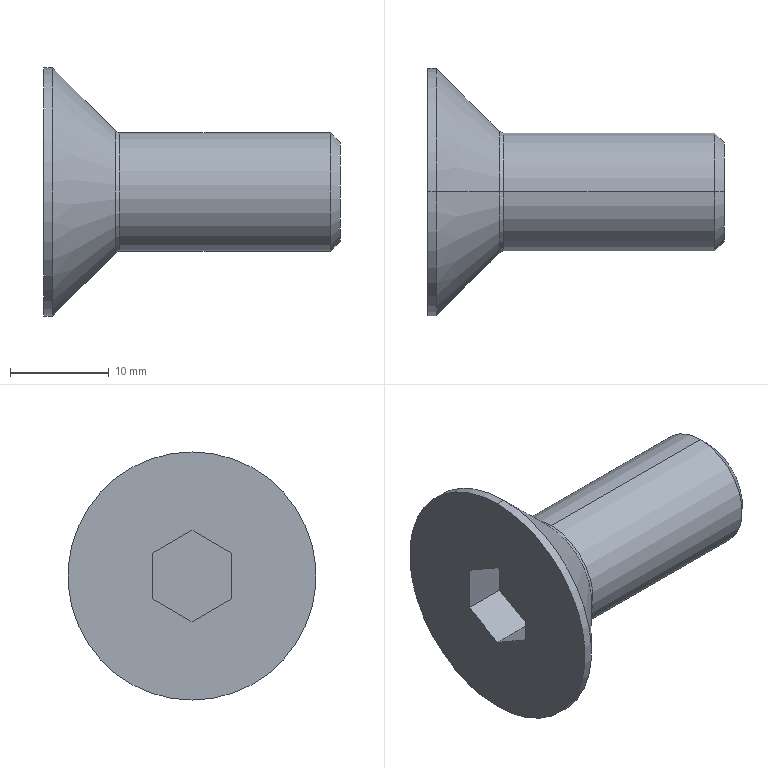Part | STEP file | 1 solid | 19 faces | box 30 x 25.075 x 25.075 mm | volume 4579 mm3 | plane 9 | cone 4 | cylinder 4 | spline 2 | commonest cylinder face diameters 12 x2 25.075 x2
STEP:
#1=CARTESIAN_POINT('',(0.,0.,0.));
#2=DIRECTION('',(0.,0.,1.));
#3=DIRECTION('',(1.,0.,0.));
#4=AXIS2_PLACEMENT_3D('',#1,#2,#3);
#5=CARTESIAN_POINT('',(22.56,0.,5.));
#6=VERTEX_POINT('',#5);
#7=CARTESIAN_POINT('',(22.56,0.,-5.));
#8=VERTEX_POINT('',#7);
#9=CARTESIAN_POINT('',(22.56,0.,0.));
#10=DIRECTION('',(-1.,0.,0.));
#11=DIRECTION('',(0.,0.,1.));
#12=AXIS2_PLACEMENT_3D('',#9,#10,#11);
#13=CIRCLE('',#12,5.);
#14=CARTESIAN_POINT('',(22.56,6.,0.));
#15=DIRECTION('',(-1.,0.,0.));
#16=DIRECTION('',(0.,0.,1.));
#17=AXIS2_PLACEMENT_3D('',#14,#15,#16);
#18=PLANE('',#17);
#19=CARTESIAN_POINT('',(0.,-6.));
#20=DIRECTION('',(1.,0.));
#21=AXIS2_PLACEMENT_2D('',#19,#20);
#22=CIRCLE('',#21,5.);
#23=(GEOMETRIC_REPRESENTATION_CONTEXT(2)PARAMETRIC_REPRESENTATION_CONTEXT()REPRESENTATION_CONTEXT('',''));
#24=DEFINITIONAL_REPRESENTATION('',(#22),#23);
#25=PCURVE('',#18,#24);
#26=CARTESIAN_POINT('',(21.56,0.,0.));
#27=DIRECTION('',(-1.,0.,0.));
#28=DIRECTION('',(0.,0.,1.));
#29=AXIS2_PLACEMENT_3D('',#26,#27,#28);
#30=CONICAL_SURFACE('',#29,6.,0.7854);
#31=CARTESIAN_POINT('',(0.,-1.));
#32=DIRECTION('',(1.,0.));
#33=VECTOR('',#32,1.);
#34=LINE('',#31,#33);
#35=(GEOMETRIC_REPRESENTATION_CONTEXT(2)PARAMETRIC_REPRESENTATION_CONTEXT()REPRESENTATION_CONTEXT('',''));
#36=DEFINITIONAL_REPRESENTATION('',(#34),#35);
#37=PCURVE('',#30,#36);
#38=SURFACE_CURVE('',#13,(#25,#37),.PCURVE_S1.);
#39=EDGE_CURVE('',#6,#8,#38,.T.);
#40=ORIENTED_EDGE('',*,*,#39,.F.);
#41=CARTESIAN_POINT('',(22.56,0.,0.));
#42=DIRECTION('',(-1.,0.,0.));
#43=DIRECTION('',(0.,0.,1.));
#44=AXIS2_PLACEMENT_3D('',#41,#42,#43);
#45=CIRCLE('',#44,5.);
#46=CARTESIAN_POINT('',(0.,-6.));
#47=DIRECTION('',(1.,0.));
#48=AXIS2_PLACEMENT_2D('',#46,#47);
#49=CIRCLE('',#48,5.);
#50=(GEOMETRIC_REPRESENTATION_CONTEXT(2)PARAMETRIC_REPRESENTATION_CONTEXT()REPRESENTATION_CONTEXT('',''));
#51=DEFINITIONAL_REPRESENTATION('',(#49),#50);
#52=PCURVE('',#18,#51);
#53=CARTESIAN_POINT('',(21.56,0.,0.));
#54=DIRECTION('',(-1.,0.,0.));
#55=DIRECTION('',(0.,0.,1.));
#56=AXIS2_PLACEMENT_3D('',#53,#54,#55);
#57=CONICAL_SURFACE('',#56,6.,0.7854);
#58=CARTESIAN_POINT('',(0.,-1.));
#59=DIRECTION('',(1.,0.));
#60=VECTOR('',#59,1.);
#61=LINE('',#58,#60);
#62=(GEOMETRIC_REPRESENTATION_CONTEXT(2)PARAMETRIC_REPRESENTATION_CONTEXT()REPRESENTATION_CONTEXT('',''));
#63=DEFINITIONAL_REPRESENTATION('',(#61),#62);
#64=PCURVE('',#57,#63);
#65=SURFACE_CURVE('',#45,(#52,#64),.PCURVE_S1.);
#66=EDGE_CURVE('',#8,#6,#65,.T.);
#67=ORIENTED_EDGE('',*,*,#66,.F.);
#68=EDGE_LOOP('',(#40,#67));
#69=FACE_BOUND('',#68,.T.);
#70=ADVANCED_FACE('',(#69),#18,.F.);
#71=CARTESIAN_POINT('',(21.56,0.,-6.));
#72=VERTEX_POINT('',#71);
#73=CARTESIAN_POINT('',(21.56,0.,-6.));
#74=DIRECTION('',(-0.7071,0.,-0.7071));
#75=VECTOR('',#74,1.);
#76=LINE('',#73,#75);
#77=CARTESIAN_POINT('',(3.142,0.));
#78=DIRECTION('',(0.,1.));
#79=VECTOR('',#78,1.);
#80=LINE('',#77,#79);
#81=(GEOMETRIC_REPRESENTATION_CONTEXT(2)PARAMETRIC_REPRESENTATION_CONTEXT()REPRESENTATION_CONTEXT('',''));
#82=DEFINITIONAL_REPRESENTATION('',(#80),#81);
#83=PCURVE('',#57,#82);
#84=CARTESIAN_POINT('',(3.142,0.));
#85=DIRECTION('',(0.,1.));
#86=VECTOR('',#85,1.);
#87=LINE('',#84,#86);
#88=(GEOMETRIC_REPRESENTATION_CONTEXT(2)PARAMETRIC_REPRESENTATION_CONTEXT()REPRESENTATION_CONTEXT('',''));
#89=DEFINITIONAL_REPRESENTATION('',(#87),#88);
#90=PCURVE('',#30,#89);
#91=SURFACE_CURVE('',#76,(#83,#90),.PCURVE_S1.);
#92=EDGE_CURVE('',#8,#72,#91,.T.);
#93=ORIENTED_EDGE('',*,*,#92,.F.);
#94=ORIENTED_EDGE('',*,*,#66,.T.);
#95=CARTESIAN_POINT('',(21.56,0.,6.));
#96=VERTEX_POINT('',#95);
#97=CARTESIAN_POINT('',(21.56,0.,6.));
#98=DIRECTION('',(-0.7071,0.,0.7071));
#99=VECTOR('',#98,1.);
#100=LINE('',#97,#99);
#101=CARTESIAN_POINT('',(6.283,0.));
#102=DIRECTION('',(0.,1.));
#103=VECTOR('',#102,1.);
#104=LINE('',#101,#103);
#105=(GEOMETRIC_REPRESENTATION_CONTEXT(2)PARAMETRIC_REPRESENTATION_CONTEXT()REPRESENTATION_CONTEXT('',''));
#106=DEFINITIONAL_REPRESENTATION('',(#104),#105);
#107=PCURVE('',#57,#106);
#108=CARTESIAN_POINT('',(0.,0.));
#109=DIRECTION('',(0.,1.));
#110=VECTOR('',#109,1.);
#111=LINE('',#108,#110);
#112=(GEOMETRIC_REPRESENTATION_CONTEXT(2)PARAMETRIC_REPRESENTATION_CONTEXT()REPRESENTATION_CONTEXT('',''));
#113=DEFINITIONAL_REPRESENTATION('',(#111),#112);
#114=PCURVE('',#30,#113);
#115=SURFACE_CURVE('',#100,(#107,#114),.PCURVE_S1.);
#116=EDGE_CURVE('',#6,#96,#115,.T.);
#117=ORIENTED_EDGE('',*,*,#116,.T.);
#118=CARTESIAN_POINT('',(21.56,0.,0.));
#119=DIRECTION('',(-1.,0.,0.));
#120=DIRECTION('',(0.,0.,1.));
#121=AXIS2_PLACEMENT_3D('',#118,#119,#120);
#122=CIRCLE('',#121,6.);
#123=CARTESIAN_POINT('',(0.,0.));
#124=DIRECTION('',(1.,0.));
#125=VECTOR('',#124,1.);
#126=LINE('',#123,#125);
#127=(GEOMETRIC_REPRESENTATION_CONTEXT(2)PARAMETRIC_REPRESENTATION_CONTEXT()REPRESENTATION_CONTEXT('',''));
#128=DEFINITIONAL_REPRESENTATION('',(#126),#127);
#129=PCURVE('',#57,#128);
#130=CARTESIAN_POINT('',(-37.991,0.,0.));
#131=DIRECTION('',(-1.,0.,0.));
#132=DIRECTION('',(0.,0.,1.));
#133=AXIS2_PLACEMENT_3D('',#130,#131,#132);
#134=CYLINDRICAL_SURFACE('',#133,6.);
#135=CARTESIAN_POINT('',(0.,-59.551));
#136=DIRECTION('',(1.,0.));
#137=VECTOR('',#136,1.);
#138=LINE('',#135,#137);
#139=(GEOMETRIC_REPRESENTATION_CONTEXT(2)PARAMETRIC_REPRESENTATION_CONTEXT()REPRESENTATION_CONTEXT('',''));
#140=DEFINITIONAL_REPRESENTATION('',(#138),#139);
#141=PCURVE('',#134,#140);
#142=SURFACE_CURVE('',#122,(#129,#141),.PCURVE_S1.);
#143=EDGE_CURVE('',#72,#96,#142,.T.);
#144=ORIENTED_EDGE('',*,*,#143,.F.);
#145=EDGE_LOOP('',(#93,#94,#117,#144));
#146=FACE_BOUND('',#145,.T.);
#147=ADVANCED_FACE('',(#146),#57,.T.);
#148=CARTESIAN_POINT('',(0.2485,0.,-6.));
#149=VERTEX_POINT('',#148);
#150=CARTESIAN_POINT('',(-37.991,0.,-6.));
#151=DIRECTION('',(-1.,0.,0.));
#152=VECTOR('',#151,1.);
#153=LINE('',#150,#152);
#154=CARTESIAN_POINT('',(3.142,0.));
#155=DIRECTION('',(0.,1.));
#156=VECTOR('',#155,1.);
#157=LINE('',#154,#156);
#158=(GEOMETRIC_REPRESENTATION_CONTEXT(2)PARAMETRIC_REPRESENTATION_CONTEXT()REPRESENTATION_CONTEXT('',''));
#159=DEFINITIONAL_REPRESENTATION('',(#157),#158);
#160=PCURVE('',#134,#159);
#161=CARTESIAN_POINT('',(-37.991,0.,0.));
#162=DIRECTION('',(-1.,0.,0.));
#163=DIRECTION('',(0.,0.,1.));
#164=AXIS2_PLACEMENT_3D('',#161,#162,#163);
#165=CYLINDRICAL_SURFACE('',#164,6.);
#166=CARTESIAN_POINT('',(3.142,0.));
#167=DIRECTION('',(0.,1.));
#168=VECTOR('',#167,1.);
#169=LINE('',#166,#168);
#170=(GEOMETRIC_REPRESENTATION_CONTEXT(2)PARAMETRIC_REPRESENTATION_CONTEXT()REPRESENTATION_CONTEXT('',''));
#171=DEFINITIONAL_REPRESENTATION('',(#169),#170);
#172=PCURVE('',#165,#171);
#173=SURFACE_CURVE('',#153,(#160,#172),.PCURVE_S1.);
#174=EDGE_CURVE('',#72,#149,#173,.T.);
#175=ORIENTED_EDGE('',*,*,#174,.F.);
#176=ORIENTED_EDGE('',*,*,#143,.T.);
#177=CARTESIAN_POINT('',(0.2485,0.,6.));
#178=VERTEX_POINT('',#177);
#179=CARTESIAN_POINT('',(-37.991,0.,6.));
#180=DIRECTION('',(-1.,0.,0.));
#181=VECTOR('',#180,1.);
#182=LINE('',#179,#181);
#183=CARTESIAN_POINT('',(6.283,0.));
#184=DIRECTION('',(0.,1.));
#185=VECTOR('',#184,1.);
#186=LINE('',#183,#185);
#187=(GEOMETRIC_REPRESENTATION_CONTEXT(2)PARAMETRIC_REPRESENTATION_CONTEXT()REPRESENTATION_CONTEXT('',''));
#188=DEFINITIONAL_REPRESENTATION('',(#186),#187);
#189=PCURVE('',#134,#188);
#190=CARTESIAN_POINT('',(0.,0.));
#191=DIRECTION('',(0.,1.));
#192=VECTOR('',#191,1.);
#193=LINE('',#190,#192);
#194=(GEOMETRIC_REPRESENTATION_CONTEXT(2)PARAMETRIC_REPRESENTATION_CONTEXT()REPRESENTATION_CONTEXT('',''));
#195=DEFINITIONAL_REPRESENTATION('',(#193),#194);
#196=PCURVE('',#165,#195);
#197=SURFACE_CURVE('',#182,(#189,#196),.PCURVE_S1.);
#198=EDGE_CURVE('',#96,#178,#197,.T.);
#199=ORIENTED_EDGE('',*,*,#198,.T.);
#200=CARTESIAN_POINT('',(0.2485,0.,0.));
#201=DIRECTION('',(1.,0.,0.));
#202=DIRECTION('',(0.,0.,1.));
#203=AXIS2_PLACEMENT_3D('',#200,#201,#202);
#204=CIRCLE('',#203,6.);
#205=CARTESIAN_POINT('',(6.283,-38.239));
#206=DIRECTION('',(-1.,0.));
#207=VECTOR('',#206,1.);
#208=LINE('',#205,#207);
#209=(GEOMETRIC_REPRESENTATION_CONTEXT(2)PARAMETRIC_REPRESENTATION_CONTEXT()REPRESENTATION_CONTEXT('',''));
#210=DEFINITIONAL_REPRESENTATION('',(#208),#209);
#211=PCURVE('',#134,#210);
#212=CARTESIAN_POINT('',(0.2485,0.,-6.));
#213=CARTESIAN_POINT('',(0.2485,-12.,-6.));
#214=CARTESIAN_POINT('',(0.2485,-12.,6.));
#215=CARTESIAN_POINT('',(0.2485,0.,6.));
#216=CARTESIAN_POINT('',(0.08727,0.,-6.));
#217=CARTESIAN_POINT('',(0.08727,-12.,-6.));
#218=CARTESIAN_POINT('',(0.08727,-12.,6.));
#219=CARTESIAN_POINT('',(0.08727,0.,6.));
#220=CARTESIAN_POINT('',(-0.06171,0.,-6.062));
#221=CARTESIAN_POINT('',(-0.06171,-12.123,-6.062));
#222=CARTESIAN_POINT('',(-0.06171,-12.123,6.062));
#223=CARTESIAN_POINT('',(-0.06171,0.,6.062));
#224=CARTESIAN_POINT('',(-0.1757,0.,-6.176));
#225=CARTESIAN_POINT('',(-0.1757,-12.351,-6.176));
#226=CARTESIAN_POINT('',(-0.1757,-12.351,6.176));
#227=CARTESIAN_POINT('',(-0.1757,0.,6.176));
#228=(BOUNDED_SURFACE()B_SPLINE_SURFACE(3,3,((#212,#213,#214,#215),(#216,#217,#218,#219),(#220,#221,#222,#223),(#224,#225,#226,#227)),.UNSPECIFIED.,.F.,.F.,.F.)B_SPLINE_SURFACE_WITH_KNOTS((4,4),(4,4),(0.,1.),(0.,1.),.PIECEWISE_BEZIER_KNOTS.)GEOMETRIC_REPRESENTATION_ITEM()RATIONAL_B_SPLINE_SURFACE(((1.,0.3333,0.3333,1.),(0.9493,0.3164,0.3164,0.9493),(0.9493,0.3164,0.3164,0.9493),(1.,0.3333,0.3333,1.)))REPRESENTATION_ITEM('')SURFACE());
#229=CARTESIAN_POINT('',(0.,1.));
#230=CARTESIAN_POINT('',(0.,0.9763));
#231=CARTESIAN_POINT('',(0.,0.9319));
#232=CARTESIAN_POINT('',(0.,0.8733));
#233=CARTESIAN_POINT('',(0.,0.8206));
#234=CARTESIAN_POINT('',(0.,0.7724));
#235=CARTESIAN_POINT('',(0.,0.7279));
#236=CARTESIAN_POINT('',(0.,0.6861));
#237=CARTESIAN_POINT('',(0.,0.6465));
#238=CARTESIAN_POINT('',(0.,0.6086));
#239=CARTESIAN_POINT('',(0.,0.5718));
#240=CARTESIAN_POINT('',(0.,0.5357));
#241=CARTESIAN_POINT('',(0.,0.5));
#242=CARTESIAN_POINT('',(0.,0.4643));
#243=CARTESIAN_POINT('',(0.,0.4282));
#244=CARTESIAN_POINT('',(0.,0.3914));
#245=CARTESIAN_POINT('',(0.,0.3535));
#246=CARTESIAN_POINT('',(0.,0.3139));
#247=CARTESIAN_POINT('',(0.,0.2721));
#248=CARTESIAN_POINT('',(0.,0.2276));
#249=CARTESIAN_POINT('',(0.,0.1794));
#250=CARTESIAN_POINT('',(0.,0.1267));
#251=CARTESIAN_POINT('',(0.,0.06805));
#252=CARTESIAN_POINT('',(0.,0.02375));
#253=CARTESIAN_POINT('',(0.,0.));
#254=B_SPLINE_CURVE_WITH_KNOTS('',3,(#229,#230,#231,#232,#233,#234,#235,#236,#237,#238,#239,#240,#241,#242,#243,#244,#245,#246,#247,#248,#249,#250,#251,#252,#253),.UNSPECIFIED.,.F.,.F.,(4,1,1,1,1,1,1,1,1,1,1,1,1,1,1,1,1,1,1,1,1,1,4),(0.,0.1428,0.2856,0.4284,0.5712,0.714,0.8568,0.9996,1.142,1.285,1.428,1.571,1.714,1.856,1.999,2.142,2.285,2.428,2.57,2.713,2.856,2.999,3.142),.QUASI_UNIFORM_KNOTS.);
#255=(GEOMETRIC_REPRESENTATION_CONTEXT(2)PARAMETRIC_REPRESENTATION_CONTEXT()REPRESENTATION_CONTEXT('',''));
#256=DEFINITIONAL_REPRESENTATION('',(#254),#255);
#257=PCURVE('',#228,#256);
#258=SURFACE_CURVE('',#204,(#211,#257),.PCURVE_S1.);
#259=EDGE_CURVE('',#178,#149,#258,.T.);
#260=ORIENTED_EDGE('',*,*,#259,.T.);
#261=EDGE_LOOP('',(#175,#176,#199,#260));
#262=FACE_BOUND('',#261,.T.);
#263=ADVANCED_FACE('',(#262),#134,.T.);
#264=CARTESIAN_POINT('',(-0.1757,0.,-6.176));
#265=VERTEX_POINT('',#264);
#266=CARTESIAN_POINT('',(-0.1757,0.,6.176));
#267=VERTEX_POINT('',#266);
#268=CARTESIAN_POINT('',(-0.1757,0.,0.));
#269=DIRECTION('',(-1.,0.,0.));
#270=DIRECTION('',(0.,0.,1.));
#271=AXIS2_PLACEMENT_3D('',#268,#269,#270);
#272=CIRCLE('',#271,6.176);
#273=CARTESIAN_POINT('',(1.,0.));
#274=CARTESIAN_POINT('',(1.,0.02375));
#275=CARTESIAN_POINT('',(1.,0.06805));
#276=CARTESIAN_POINT('',(1.,0.1267));
#277=CARTESIAN_POINT('',(1.,0.1794));
#278=CARTESIAN_POINT('',(1.,0.2276));
#279=CARTESIAN_POINT('',(1.,0.2721));
#280=CARTESIAN_POINT('',(1.,0.3139));
#281=CARTESIAN_POINT('',(1.,0.3535));
#282=CARTESIAN_POINT('',(1.,0.3914));
#283=CARTESIAN_POINT('',(1.,0.4282));
#284=CARTESIAN_POINT('',(1.,0.4643));
#285=CARTESIAN_POINT('',(1.,0.5));
#286=CARTESIAN_POINT('',(1.,0.5357));
#287=CARTESIAN_POINT('',(1.,0.5718));
#288=CARTESIAN_POINT('',(1.,0.6086));
#289=CARTESIAN_POINT('',(1.,0.6465));
#290=CARTESIAN_POINT('',(1.,0.6861));
#291=CARTESIAN_POINT('',(1.,0.7279));
#292=CARTESIAN_POINT('',(1.,0.7724));
#293=CARTESIAN_POINT('',(1.,0.8206));
#294=CARTESIAN_POINT('',(1.,0.8733));
#295=CARTESIAN_POINT('',(1.,0.9319));
#296=CARTESIAN_POINT('',(1.,0.9763));
#297=CARTESIAN_POINT('',(1.,1.));
#298=B_SPLINE_CURVE_WITH_KNOTS('',3,(#273,#274,#275,#276,#277,#278,#279,#280,#281,#282,#283,#284,#285,#286,#287,#288,#289,#290,#291,#292,#293,#294,#295,#296,#297),.UNSPECIFIED.,.F.,.F.,(4,1,1,1,1,1,1,1,1,1,1,1,1,1,1,1,1,1,1,1,1,1,4),(3.142,3.284,3.427,3.57,3.713,3.856,3.998,4.141,4.284,4.427,4.57,4.712,4.855,4.998,5.141,5.284,5.426,5.569,5.712,5.855,5.998,6.14,6.283),.QUASI_UNIFORM_KNOTS.);
#299=(GEOMETRIC_REPRESENTATION_CONTEXT(2)PARAMETRIC_REPRESENTATION_CONTEXT()REPRESENTATION_CONTEXT('',''));
#300=DEFINITIONAL_REPRESENTATION('',(#298),#299);
#301=PCURVE('',#228,#300);
#302=CARTESIAN_POINT('',(-6.537,0.,0.));
#303=DIRECTION('',(-1.,0.,0.));
#304=DIRECTION('',(0.,0.,1.));
#305=AXIS2_PLACEMENT_3D('',#302,#303,#304);
#306=CONICAL_SURFACE('',#305,12.537,0.7854);
#307=CARTESIAN_POINT('',(0.,-6.362));
#308=DIRECTION('',(1.,0.));
#309=VECTOR('',#308,1.);
#310=LINE('',#307,#309);
#311=(GEOMETRIC_REPRESENTATION_CONTEXT(2)PARAMETRIC_REPRESENTATION_CONTEXT()REPRESENTATION_CONTEXT('',''));
#312=DEFINITIONAL_REPRESENTATION('',(#310),#311);
#313=PCURVE('',#306,#312);
#314=SURFACE_CURVE('',#272,(#301,#313),.PCURVE_S1.);
#315=EDGE_CURVE('',#265,#267,#314,.T.);
#316=ORIENTED_EDGE('',*,*,#315,.T.);
#317=CARTESIAN_POINT('',(0.2485,0.,6.6));
#318=DIRECTION('',(0.,1.,0.));
#319=DIRECTION('',(0.,0.,1.));
#320=AXIS2_PLACEMENT_3D('',#317,#318,#319);
#321=CIRCLE('',#320,0.6);
#322=CARTESIAN_POINT('',(0.,1.));
#323=CARTESIAN_POINT('',(0.01555,1.));
#324=CARTESIAN_POINT('',(0.04653,1.));
#325=CARTESIAN_POINT('',(0.09271,1.));
#326=CARTESIAN_POINT('',(0.1386,1.));
#327=CARTESIAN_POINT('',(0.1843,1.));
#328=CARTESIAN_POINT('',(0.2298,1.));
#329=CARTESIAN_POINT('',(0.2751,1.));
#330=CARTESIAN_POINT('',(0.3202,1.));
#331=CARTESIAN_POINT('',(0.3653,1.));
#332=CARTESIAN_POINT('',(0.4102,1.));
#333=CARTESIAN_POINT('',(0.4551,1.));
#334=CARTESIAN_POINT('',(0.5,1.));
#335=CARTESIAN_POINT('',(0.5449,1.));
#336=CARTESIAN_POINT('',(0.5898,1.));
#337=CARTESIAN_POINT('',(0.6347,1.));
#338=CARTESIAN_POINT('',(0.6798,1.));
#339=CARTESIAN_POINT('',(0.7249,1.));
#340=CARTESIAN_POINT('',(0.7702,1.));
#341=CARTESIAN_POINT('',(0.8157,1.));
#342=CARTESIAN_POINT('',(0.8614,1.));
#343=CARTESIAN_POINT('',(0.9073,1.));
#344=CARTESIAN_POINT('',(0.9535,1.));
#345=CARTESIAN_POINT('',(0.9845,1.));
#346=CARTESIAN_POINT('',(1.,1.));
#347=B_SPLINE_CURVE_WITH_KNOTS('',3,(#322,#323,#324,#325,#326,#327,#328,#329,#330,#331,#332,#333,#334,#335,#336,#337,#338,#339,#340,#341,#342,#343,#344,#345,#346),.UNSPECIFIED.,.F.,.F.,(4,1,1,1,1,1,1,1,1,1,1,1,1,1,1,1,1,1,1,1,1,1,4),(3.142,3.177,3.213,3.249,3.284,3.32,3.356,3.391,3.427,3.463,3.499,3.534,3.57,3.606,3.641,3.677,3.713,3.748,3.784,3.82,3.856,3.891,3.927),.QUASI_UNIFORM_KNOTS.);
#348=(GEOMETRIC_REPRESENTATION_CONTEXT(2)PARAMETRIC_REPRESENTATION_CONTEXT()REPRESENTATION_CONTEXT('',''));
#349=DEFINITIONAL_REPRESENTATION('',(#347),#348);
#350=PCURVE('',#228,#349);
#351=CARTESIAN_POINT('',(0.2485,0.,6.));
#352=CARTESIAN_POINT('',(0.2485,12.,6.));
#353=CARTESIAN_POINT('',(0.2485,12.,-6.));
#354=CARTESIAN_POINT('',(0.2485,0.,-6.));
#355=CARTESIAN_POINT('',(0.08727,0.,6.));
#356=CARTESIAN_POINT('',(0.08727,12.,6.));
#357=CARTESIAN_POINT('',(0.08727,12.,-6.));
#358=CARTESIAN_POINT('',(0.08727,0.,-6.));
#359=CARTESIAN_POINT('',(-0.06171,0.,6.062));
#360=CARTESIAN_POINT('',(-0.06171,12.123,6.062));
#361=CARTESIAN_POINT('',(-0.06171,12.123,-6.062));
#362=CARTESIAN_POINT('',(-0.06171,0.,-6.062));
#363=CARTESIAN_POINT('',(-0.1757,0.,6.176));
#364=CARTESIAN_POINT('',(-0.1757,12.351,6.176));
#365=CARTESIAN_POINT('',(-0.1757,12.351,-6.176));
#366=CARTESIAN_POINT('',(-0.1757,0.,-6.176));
#367=(BOUNDED_SURFACE()B_SPLINE_SURFACE(3,3,((#351,#352,#353,#354),(#355,#356,#357,#358),(#359,#360,#361,#362),(#363,#364,#365,#366)),.UNSPECIFIED.,.F.,.F.,.F.)B_SPLINE_SURFACE_WITH_KNOTS((4,4),(4,4),(0.,1.),(0.,1.),.PIECEWISE_BEZIER_KNOTS.)GEOMETRIC_REPRESENTATION_ITEM()RATIONAL_B_SPLINE_SURFACE(((1.,0.3333,0.3333,1.),(0.9493,0.3164,0.3164,0.9493),(0.9493,0.3164,0.3164,0.9493),(1.,0.3333,0.3333,1.)))REPRESENTATION_ITEM('')SURFACE());
#368=CARTESIAN_POINT('',(0.,0.));
#369=CARTESIAN_POINT('',(0.01555,0.));
#370=CARTESIAN_POINT('',(0.04653,0.));
#371=CARTESIAN_POINT('',(0.09271,0.));
#372=CARTESIAN_POINT('',(0.1386,0.));
#373=CARTESIAN_POINT('',(0.1843,0.));
#374=CARTESIAN_POINT('',(0.2298,0.));
#375=CARTESIAN_POINT('',(0.2751,0.));
#376=CARTESIAN_POINT('',(0.3202,0.));
#377=CARTESIAN_POINT('',(0.3653,0.));
#378=CARTESIAN_POINT('',(0.4102,0.));
#379=CARTESIAN_POINT('',(0.4551,0.));
#380=CARTESIAN_POINT('',(0.5,0.));
#381=CARTESIAN_POINT('',(0.5449,0.));
#382=CARTESIAN_POINT('',(0.5898,0.));
#383=CARTESIAN_POINT('',(0.6347,0.));
#384=CARTESIAN_POINT('',(0.6798,0.));
#385=CARTESIAN_POINT('',(0.7249,0.));
#386=CARTESIAN_POINT('',(0.7702,0.));
#387=CARTESIAN_POINT('',(0.8157,0.));
#388=CARTESIAN_POINT('',(0.8614,0.));
#389=CARTESIAN_POINT('',(0.9073,0.));
#390=CARTESIAN_POINT('',(0.9535,0.));
#391=CARTESIAN_POINT('',(0.9845,0.));
#392=CARTESIAN_POINT('',(1.,0.));
#393=B_SPLINE_CURVE_WITH_KNOTS('',3,(#368,#369,#370,#371,#372,#373,#374,#375,#376,#377,#378,#379,#380,#381,#382,#383,#384,#385,#386,#387,#388,#389,#390,#391,#392),.UNSPECIFIED.,.F.,.F.,(4,1,1,1,1,1,1,1,1,1,1,1,1,1,1,1,1,1,1,1,1,1,4),(3.142,3.177,3.213,3.249,3.284,3.32,3.356,3.391,3.427,3.463,3.499,3.534,3.57,3.606,3.641,3.677,3.713,3.748,3.784,3.82,3.856,3.891,3.927),.QUASI_UNIFORM_KNOTS.);
#394=(GEOMETRIC_REPRESENTATION_CONTEXT(2)PARAMETRIC_REPRESENTATION_CONTEXT()REPRESENTATION_CONTEXT('',''));
#395=DEFINITIONAL_REPRESENTATION('',(#393),#394);
#396=PCURVE('',#367,#395);
#397=SURFACE_CURVE('',#321,(#350,#396),.PCURVE_S1.);
#398=EDGE_CURVE('',#178,#267,#397,.T.);
#399=ORIENTED_EDGE('',*,*,#398,.F.);
#400=ORIENTED_EDGE('',*,*,#259,.T.);
#401=CARTESIAN_POINT('',(0.2485,0.,-6.6));
#402=DIRECTION('',(0.,-1.,0.));
#403=DIRECTION('',(0.,0.,-1.));
#404=AXIS2_PLACEMENT_3D('',#401,#402,#403);
#405=CIRCLE('',#404,0.6);
#406=CARTESIAN_POINT('',(0.,0.));
#407=CARTESIAN_POINT('',(0.01555,0.));
#408=CARTESIAN_POINT('',(0.04653,0.));
#409=CARTESIAN_POINT('',(0.09271,0.));
#410=CARTESIAN_POINT('',(0.1386,0.));
#411=CARTESIAN_POINT('',(0.1843,0.));
#412=CARTESIAN_POINT('',(0.2298,0.));
#413=CARTESIAN_POINT('',(0.2751,0.));
#414=CARTESIAN_POINT('',(0.3202,0.));
#415=CARTESIAN_POINT('',(0.3653,0.));
#416=CARTESIAN_POINT('',(0.4102,0.));
#417=CARTESIAN_POINT('',(0.4551,0.));
#418=CARTESIAN_POINT('',(0.5,0.));
#419=CARTESIAN_POINT('',(0.5449,0.));
#420=CARTESIAN_POINT('',(0.5898,0.));
#421=CARTESIAN_POINT('',(0.6347,0.));
#422=CARTESIAN_POINT('',(0.6798,0.));
#423=CARTESIAN_POINT('',(0.7249,0.));
#424=CARTESIAN_POINT('',(0.7702,0.));
#425=CARTESIAN_POINT('',(0.8157,0.));
#426=CARTESIAN_POINT('',(0.8614,0.));
#427=CARTESIAN_POINT('',(0.9073,0.));
#428=CARTESIAN_POINT('',(0.9535,0.));
#429=CARTESIAN_POINT('',(0.9845,0.));
#430=CARTESIAN_POINT('',(1.,0.));
#431=B_SPLINE_CURVE_WITH_KNOTS('',3,(#406,#407,#408,#409,#410,#411,#412,#413,#414,#415,#416,#417,#418,#419,#420,#421,#422,#423,#424,#425,#426,#427,#428,#429,#430),.UNSPECIFIED.,.F.,.F.,(4,1,1,1,1,1,1,1,1,1,1,1,1,1,1,1,1,1,1,1,1,1,4),(3.142,3.177,3.213,3.249,3.284,3.32,3.356,3.391,3.427,3.463,3.499,3.534,3.57,3.606,3.641,3.677,3.713,3.748,3.784,3.82,3.856,3.891,3.927),.QUASI_UNIFORM_KNOTS.);
#432=(GEOMETRIC_REPRESENTATION_CONTEXT(2)PARAMETRIC_REPRESENTATION_CONTEXT()REPRESENTATION_CONTEXT('',''));
#433=DEFINITIONAL_REPRESENTATION('',(#431),#432);
#434=PCURVE('',#228,#433);
#435=CARTESIAN_POINT('',(0.,1.));
#436=CARTESIAN_POINT('',(0.01555,1.));
#437=CARTESIAN_POINT('',(0.04653,1.));
#438=CARTESIAN_POINT('',(0.09271,1.));
#439=CARTESIAN_POINT('',(0.1386,1.));
#440=CARTESIAN_POINT('',(0.1843,1.));
#441=CARTESIAN_POINT('',(0.2298,1.));
#442=CARTESIAN_POINT('',(0.2751,1.));
#443=CARTESIAN_POINT('',(0.3202,1.));
#444=CARTESIAN_POINT('',(0.3653,1.));
#445=CARTESIAN_POINT('',(0.4102,1.));
#446=CARTESIAN_POINT('',(0.4551,1.));
#447=CARTESIAN_POINT('',(0.5,1.));
#448=CARTESIAN_POINT('',(0.5449,1.));
#449=CARTESIAN_POINT('',(0.5898,1.));
#450=CARTESIAN_POINT('',(0.6347,1.));
#451=CARTESIAN_POINT('',(0.6798,1.));
#452=CARTESIAN_POINT('',(0.7249,1.));
#453=CARTESIAN_POINT('',(0.7702,1.));
#454=CARTESIAN_POINT('',(0.8157,1.));
#455=CARTESIAN_POINT('',(0.8614,1.));
#456=CARTESIAN_POINT('',(0.9073,1.));
#457=CARTESIAN_POINT('',(0.9535,1.));
#458=CARTESIAN_POINT('',(0.9845,1.));
#459=CARTESIAN_POINT('',(1.,1.));
#460=B_SPLINE_CURVE_WITH_KNOTS('',3,(#435,#436,#437,#438,#439,#440,#441,#442,#443,#444,#445,#446,#447,#448,#449,#450,#451,#452,#453,#454,#455,#456,#457,#458,#459),.UNSPECIFIED.,.F.,.F.,(4,1,1,1,1,1,1,1,1,1,1,1,1,1,1,1,1,1,1,1,1,1,4),(3.142,3.177,3.213,3.249,3.284,3.32,3.356,3.391,3.427,3.463,3.499,3.534,3.57,3.606,3.641,3.677,3.713,3.748,3.784,3.82,3.856,3.891,3.927),.QUASI_UNIFORM_KNOTS.);
#461=(GEOMETRIC_REPRESENTATION_CONTEXT(2)PARAMETRIC_REPRESENTATION_CONTEXT()REPRESENTATION_CONTEXT('',''));
#462=DEFINITIONAL_REPRESENTATION('',(#460),#461);
#463=PCURVE('',#367,#462);
#464=SURFACE_CURVE('',#405,(#434,#463),.PCURVE_S1.);
#465=EDGE_CURVE('',#149,#265,#464,.T.);
#466=ORIENTED_EDGE('',*,*,#465,.T.);
#467=EDGE_LOOP('',(#316,#399,#400,#466));
#468=FACE_BOUND('',#467,.F.);
#469=ADVANCED_FACE('',(#468),#228,.F.);
#470=CARTESIAN_POINT('',(-3.14,-4.,-2.309));
#471=VERTEX_POINT('',#470);
#472=CARTESIAN_POINT('',(-3.14,-4.,2.309));
#473=VERTEX_POINT('',#472);
#474=CARTESIAN_POINT('',(-3.14,-4.,-2.309));
#475=DIRECTION('',(0.,0.,1.));
#476=VECTOR('',#475,1.);
#477=LINE('',#474,#476);
#478=CARTESIAN_POINT('',(-3.14,0.,0.));
#479=DIRECTION('',(-1.,0.,0.));
#480=DIRECTION('',(0.,0.,1.));
#481=AXIS2_PLACEMENT_3D('',#478,#479,#480);
#482=PLANE('',#481);
#483=CARTESIAN_POINT('',(-2.309,-4.));
#484=DIRECTION('',(1.,0.));
#485=VECTOR('',#484,1.);
#486=LINE('',#483,#485);
#487=(GEOMETRIC_REPRESENTATION_CONTEXT(2)PARAMETRIC_REPRESENTATION_CONTEXT()REPRESENTATION_CONTEXT('',''));
#488=DEFINITIONAL_REPRESENTATION('',(#486),#487);
#489=PCURVE('',#482,#488);
#490=CARTESIAN_POINT('',(-3.14,-4.,-2.309));
#491=DIRECTION('',(0.,-1.,0.));
#492=DIRECTION('',(-1.,0.,0.));
#493=AXIS2_PLACEMENT_3D('',#490,#491,#492);
#494=PLANE('',#493);
#495=CARTESIAN_POINT('',(0.,0.));
#496=DIRECTION('',(0.,-1.));
#497=VECTOR('',#496,1.);
#498=LINE('',#495,#497);
#499=(GEOMETRIC_REPRESENTATION_CONTEXT(2)PARAMETRIC_REPRESENTATION_CONTEXT()REPRESENTATION_CONTEXT('',''));
#500=DEFINITIONAL_REPRESENTATION('',(#498),#499);
#501=PCURVE('',#494,#500);
#502=SURFACE_CURVE('',#477,(#489,#501),.PCURVE_S1.);
#503=EDGE_CURVE('',#471,#473,#502,.T.);
#504=ORIENTED_EDGE('',*,*,#503,.T.);
#505=CARTESIAN_POINT('',(-3.14,0.,4.619));
#506=VERTEX_POINT('',#505);
#507=CARTESIAN_POINT('',(-3.14,-4.,2.309));
#508=DIRECTION('',(0.,0.866,0.5));
#509=VECTOR('',#508,1.);
#510=LINE('',#507,#509);
#511=CARTESIAN_POINT('',(2.309,-4.));
#512=DIRECTION('',(0.5,0.866));
#513=VECTOR('',#512,1.);
#514=LINE('',#511,#513);
#515=(GEOMETRIC_REPRESENTATION_CONTEXT(2)PARAMETRIC_REPRESENTATION_CONTEXT()REPRESENTATION_CONTEXT('',''));
#516=DEFINITIONAL_REPRESENTATION('',(#514),#515);
#517=PCURVE('',#482,#516);
#518=CARTESIAN_POINT('',(-3.14,-4.,2.309));
#519=DIRECTION('',(0.,-0.5,0.866));
#520=DIRECTION('',(-1.,0.,0.));
#521=AXIS2_PLACEMENT_3D('',#518,#519,#520);
#522=PLANE('',#521);
#523=CARTESIAN_POINT('',(0.,0.));
#524=DIRECTION('',(0.,-1.));
#525=VECTOR('',#524,1.);
#526=LINE('',#523,#525);
#527=(GEOMETRIC_REPRESENTATION_CONTEXT(2)PARAMETRIC_REPRESENTATION_CONTEXT()REPRESENTATION_CONTEXT('',''));
#528=DEFINITIONAL_REPRESENTATION('',(#526),#527);
#529=PCURVE('',#522,#528);
#530=SURFACE_CURVE('',#510,(#517,#529),.PCURVE_S1.);
#531=EDGE_CURVE('',#473,#506,#530,.T.);
#532=ORIENTED_EDGE('',*,*,#531,.T.);
#533=CARTESIAN_POINT('',(-3.14,4.,2.309));
#534=VERTEX_POINT('',#533);
#535=CARTESIAN_POINT('',(-3.14,0.,4.619));
#536=DIRECTION('',(0.,0.866,-0.5));
#537=VECTOR('',#536,1.);
#538=LINE('',#535,#537);
#539=CARTESIAN_POINT('',(4.619,0.));
#540=DIRECTION('',(-0.5,0.866));
#541=VECTOR('',#540,1.);
#542=LINE('',#539,#541);
#543=(GEOMETRIC_REPRESENTATION_CONTEXT(2)PARAMETRIC_REPRESENTATION_CONTEXT()REPRESENTATION_CONTEXT('',''));
#544=DEFINITIONAL_REPRESENTATION('',(#542),#543);
#545=PCURVE('',#482,#544);
#546=CARTESIAN_POINT('',(-3.14,0.,4.619));
#547=DIRECTION('',(0.,0.5,0.866));
#548=DIRECTION('',(1.,0.,0.));
#549=AXIS2_PLACEMENT_3D('',#546,#547,#548);
#550=PLANE('',#549);
#551=CARTESIAN_POINT('',(0.,0.));
#552=DIRECTION('',(0.,1.));
#553=VECTOR('',#552,1.);
#554=LINE('',#551,#553);
#555=(GEOMETRIC_REPRESENTATION_CONTEXT(2)PARAMETRIC_REPRESENTATION_CONTEXT()REPRESENTATION_CONTEXT('',''));
#556=DEFINITIONAL_REPRESENTATION('',(#554),#555);
#557=PCURVE('',#550,#556);
#558=SURFACE_CURVE('',#538,(#545,#557),.PCURVE_S1.);
#559=EDGE_CURVE('',#506,#534,#558,.T.);
#560=ORIENTED_EDGE('',*,*,#559,.T.);
#561=CARTESIAN_POINT('',(-3.14,4.,-2.309));
#562=VERTEX_POINT('',#561);
#563=CARTESIAN_POINT('',(-3.14,4.,2.309));
#564=DIRECTION('',(0.,0.,-1.));
#565=VECTOR('',#564,1.);
#566=LINE('',#563,#565);
#567=CARTESIAN_POINT('',(2.309,4.));
#568=DIRECTION('',(-1.,0.));
#569=VECTOR('',#568,1.);
#570=LINE('',#567,#569);
#571=(GEOMETRIC_REPRESENTATION_CONTEXT(2)PARAMETRIC_REPRESENTATION_CONTEXT()REPRESENTATION_CONTEXT('',''));
#572=DEFINITIONAL_REPRESENTATION('',(#570),#571);
#573=PCURVE('',#482,#572);
#574=CARTESIAN_POINT('',(-3.14,4.,2.309));
#575=DIRECTION('',(0.,1.,0.));
#576=DIRECTION('',(1.,0.,0.));
#577=AXIS2_PLACEMENT_3D('',#574,#575,#576);
#578=PLANE('',#577);
#579=CARTESIAN_POINT('',(0.,0.));
#580=DIRECTION('',(0.,1.));
#581=VECTOR('',#580,1.);
#582=LINE('',#579,#581);
#583=(GEOMETRIC_REPRESENTATION_CONTEXT(2)PARAMETRIC_REPRESENTATION_CONTEXT()REPRESENTATION_CONTEXT('',''));
#584=DEFINITIONAL_REPRESENTATION('',(#582),#583);
#585=PCURVE('',#578,#584);
#586=SURFACE_CURVE('',#566,(#573,#585),.PCURVE_S1.);
#587=EDGE_CURVE('',#534,#562,#586,.T.);
#588=ORIENTED_EDGE('',*,*,#587,.T.);
#589=CARTESIAN_POINT('',(-3.14,0.,-4.619));
#590=VERTEX_POINT('',#589);
#591=CARTESIAN_POINT('',(-3.14,4.,-2.309));
#592=DIRECTION('',(0.,-0.866,-0.5));
#593=VECTOR('',#592,1.);
#594=LINE('',#591,#593);
#595=CARTESIAN_POINT('',(-2.309,4.));
#596=DIRECTION('',(-0.5,-0.866));
#597=VECTOR('',#596,1.);
#598=LINE('',#595,#597);
#599=(GEOMETRIC_REPRESENTATION_CONTEXT(2)PARAMETRIC_REPRESENTATION_CONTEXT()REPRESENTATION_CONTEXT('',''));
#600=DEFINITIONAL_REPRESENTATION('',(#598),#599);
#601=PCURVE('',#482,#600);
#602=CARTESIAN_POINT('',(-3.14,4.,-2.309));
#603=DIRECTION('',(0.,0.5,-0.866));
#604=DIRECTION('',(-1.,0.,0.));
#605=AXIS2_PLACEMENT_3D('',#602,#603,#604);
#606=PLANE('',#605);
#607=CARTESIAN_POINT('',(0.,0.));
#608=DIRECTION('',(0.,-1.));
#609=VECTOR('',#608,1.);
#610=LINE('',#607,#609);
#611=(GEOMETRIC_REPRESENTATION_CONTEXT(2)PARAMETRIC_REPRESENTATION_CONTEXT()REPRESENTATION_CONTEXT('',''));
#612=DEFINITIONAL_REPRESENTATION('',(#610),#611);
#613=PCURVE('',#606,#612);
#614=SURFACE_CURVE('',#594,(#601,#613),.PCURVE_S1.);
#615=EDGE_CURVE('',#562,#590,#614,.T.);
#616=ORIENTED_EDGE('',*,*,#615,.T.);
#617=CARTESIAN_POINT('',(-3.14,0.,-4.619));
#618=DIRECTION('',(0.,-0.866,0.5));
#619=VECTOR('',#618,1.);
#620=LINE('',#617,#619);
#621=CARTESIAN_POINT('',(-4.619,0.));
#622=DIRECTION('',(0.5,-0.866));
#623=VECTOR('',#622,1.);
#624=LINE('',#621,#623);
#625=(GEOMETRIC_REPRESENTATION_CONTEXT(2)PARAMETRIC_REPRESENTATION_CONTEXT()REPRESENTATION_CONTEXT('',''));
#626=DEFINITIONAL_REPRESENTATION('',(#624),#625);
#627=PCURVE('',#482,#626);
#628=CARTESIAN_POINT('',(-3.14,0.,-4.619));
#629=DIRECTION('',(0.,-0.5,-0.866));
#630=DIRECTION('',(0.,-0.866,0.5));
#631=AXIS2_PLACEMENT_3D('',#628,#629,#630);
#632=PLANE('',#631);
#633=CARTESIAN_POINT('',(0.,0.));
#634=DIRECTION('',(1.,0.));
#635=VECTOR('',#634,1.);
#636=LINE('',#633,#635);
#637=(GEOMETRIC_REPRESENTATION_CONTEXT(2)PARAMETRIC_REPRESENTATION_CONTEXT()REPRESENTATION_CONTEXT('',''));
#638=DEFINITIONAL_REPRESENTATION('',(#636),#637);
#639=PCURVE('',#632,#638);
#640=SURFACE_CURVE('',#620,(#627,#639),.PCURVE_S1.);
#641=EDGE_CURVE('',#590,#471,#640,.T.);
#642=ORIENTED_EDGE('',*,*,#641,.T.);
#643=EDGE_LOOP('',(#504,#532,#560,#588,#616,#642));
#644=FACE_BOUND('',#643,.T.);
#645=ADVANCED_FACE('',(#644),#482,.T.);
#646=CARTESIAN_POINT('',(-6.537,0.,-12.537));
#647=VERTEX_POINT('',#646);
#648=CARTESIAN_POINT('',(-6.537,0.,-12.537));
#649=DIRECTION('',(-0.7071,0.,-0.7071));
#650=VECTOR('',#649,1.);
#651=LINE('',#648,#650);
#652=CARTESIAN_POINT('',(3.142,0.));
#653=DIRECTION('',(0.,1.));
#654=VECTOR('',#653,1.);
#655=LINE('',#652,#654);
#656=(GEOMETRIC_REPRESENTATION_CONTEXT(2)PARAMETRIC_REPRESENTATION_CONTEXT()REPRESENTATION_CONTEXT('',''));
#657=DEFINITIONAL_REPRESENTATION('',(#655),#656);
#658=PCURVE('',#306,#657);
#659=CARTESIAN_POINT('',(-6.537,0.,0.));
#660=DIRECTION('',(-1.,0.,0.));
#661=DIRECTION('',(0.,0.,1.));
#662=AXIS2_PLACEMENT_3D('',#659,#660,#661);
#663=CONICAL_SURFACE('',#662,12.537,0.7854);
#664=CARTESIAN_POINT('',(3.142,0.));
#665=DIRECTION('',(0.,1.));
#666=VECTOR('',#665,1.);
#667=LINE('',#664,#666);
#668=(GEOMETRIC_REPRESENTATION_CONTEXT(2)PARAMETRIC_REPRESENTATION_CONTEXT()REPRESENTATION_CONTEXT('',''));
#669=DEFINITIONAL_REPRESENTATION('',(#667),#668);
#670=PCURVE('',#663,#669);
#671=SURFACE_CURVE('',#651,(#658,#670),.PCURVE_S1.);
#672=EDGE_CURVE('',#265,#647,#671,.T.);
#673=ORIENTED_EDGE('',*,*,#672,.F.);
#674=ORIENTED_EDGE('',*,*,#315,.T.);
#675=CARTESIAN_POINT('',(-6.537,0.,12.537));
#676=VERTEX_POINT('',#675);
#677=CARTESIAN_POINT('',(-6.537,0.,12.537));
#678=DIRECTION('',(-0.7071,0.,0.7071));
#679=VECTOR('',#678,1.);
#680=LINE('',#677,#679);
#681=CARTESIAN_POINT('',(6.283,0.));
#682=DIRECTION('',(0.,1.));
#683=VECTOR('',#682,1.);
#684=LINE('',#681,#683);
#685=(GEOMETRIC_REPRESENTATION_CONTEXT(2)PARAMETRIC_REPRESENTATION_CONTEXT()REPRESENTATION_CONTEXT('',''));
#686=DEFINITIONAL_REPRESENTATION('',(#684),#685);
#687=PCURVE('',#306,#686);
#688=CARTESIAN_POINT('',(0.,0.));
#689=DIRECTION('',(0.,1.));
#690=VECTOR('',#689,1.);
#691=LINE('',#688,#690);
#692=(GEOMETRIC_REPRESENTATION_CONTEXT(2)PARAMETRIC_REPRESENTATION_CONTEXT()REPRESENTATION_CONTEXT('',''));
#693=DEFINITIONAL_REPRESENTATION('',(#691),#692);
#694=PCURVE('',#663,#693);
#695=SURFACE_CURVE('',#680,(#687,#694),.PCURVE_S1.);
#696=EDGE_CURVE('',#267,#676,#695,.T.);
#697=ORIENTED_EDGE('',*,*,#696,.T.);
#698=CARTESIAN_POINT('',(-6.537,0.,0.));
#699=DIRECTION('',(-1.,0.,0.));
#700=DIRECTION('',(0.,0.,1.));
#701=AXIS2_PLACEMENT_3D('',#698,#699,#700);
#702=CIRCLE('',#701,12.537);
#703=CARTESIAN_POINT('',(0.,0.));
#704=DIRECTION('',(1.,0.));
#705=VECTOR('',#704,1.);
#706=LINE('',#703,#705);
#707=(GEOMETRIC_REPRESENTATION_CONTEXT(2)PARAMETRIC_REPRESENTATION_CONTEXT()REPRESENTATION_CONTEXT('',''));
#708=DEFINITIONAL_REPRESENTATION('',(#706),#707);
#709=PCURVE('',#306,#708);
#710=CARTESIAN_POINT('',(-37.991,0.,0.));
#711=DIRECTION('',(-1.,0.,0.));
#712=DIRECTION('',(0.,0.,1.));
#713=AXIS2_PLACEMENT_3D('',#710,#711,#712);
#714=CYLINDRICAL_SURFACE('',#713,12.537);
#715=CARTESIAN_POINT('',(0.,-31.454));
#716=DIRECTION('',(1.,0.));
#717=VECTOR('',#716,1.);
#718=LINE('',#715,#717);
#719=(GEOMETRIC_REPRESENTATION_CONTEXT(2)PARAMETRIC_REPRESENTATION_CONTEXT()REPRESENTATION_CONTEXT('',''));
#720=DEFINITIONAL_REPRESENTATION('',(#718),#719);
#721=PCURVE('',#714,#720);
#722=SURFACE_CURVE('',#702,(#709,#721),.PCURVE_S1.);
#723=EDGE_CURVE('',#647,#676,#722,.T.);
#724=ORIENTED_EDGE('',*,*,#723,.F.);
#725=EDGE_LOOP('',(#673,#674,#697,#724));
#726=FACE_BOUND('',#725,.T.);
#727=ADVANCED_FACE('',(#726),#306,.T.);
#728=CARTESIAN_POINT('',(-7.44,0.,-4.619));
#729=VERTEX_POINT('',#728);
#730=CARTESIAN_POINT('',(-3.14,0.,-4.619));
#731=DIRECTION('',(1.,0.,0.));
#732=VECTOR('',#731,1.);
#733=LINE('',#730,#732);
#734=CARTESIAN_POINT('',(0.,-4.619));
#735=DIRECTION('',(-1.,0.));
#736=VECTOR('',#735,1.);
#737=LINE('',#734,#736);
#738=(GEOMETRIC_REPRESENTATION_CONTEXT(2)PARAMETRIC_REPRESENTATION_CONTEXT()REPRESENTATION_CONTEXT('',''));
#739=DEFINITIONAL_REPRESENTATION('',(#737),#738);
#740=PCURVE('',#606,#739);
#741=CARTESIAN_POINT('',(0.,0.));
#742=DIRECTION('',(0.,-1.));
#743=VECTOR('',#742,1.);
#744=LINE('',#741,#743);
#745=(GEOMETRIC_REPRESENTATION_CONTEXT(2)PARAMETRIC_REPRESENTATION_CONTEXT()REPRESENTATION_CONTEXT('',''));
#746=DEFINITIONAL_REPRESENTATION('',(#744),#745);
#747=PCURVE('',#632,#746);
#748=SURFACE_CURVE('',#733,(#740,#747),.PCURVE_S1.);
#749=EDGE_CURVE('',#729,#590,#748,.T.);
#750=ORIENTED_EDGE('',*,*,#749,.T.);
#751=ORIENTED_EDGE('',*,*,#615,.F.);
#752=CARTESIAN_POINT('',(-7.44,4.,-2.309));
#753=VERTEX_POINT('',#752);
#754=CARTESIAN_POINT('',(-3.14,4.,-2.309));
#755=DIRECTION('',(-1.,0.,0.));
#756=VECTOR('',#755,1.);
#757=LINE('',#754,#756);
#758=CARTESIAN_POINT('',(0.,0.));
#759=DIRECTION('',(1.,0.));
#760=VECTOR('',#759,1.);
#761=LINE('',#758,#760);
#762=(GEOMETRIC_REPRESENTATION_CONTEXT(2)PARAMETRIC_REPRESENTATION_CONTEXT()REPRESENTATION_CONTEXT('',''));
#763=DEFINITIONAL_REPRESENTATION('',(#761),#762);
#764=PCURVE('',#606,#763);
#765=CARTESIAN_POINT('',(0.,4.619));
#766=DIRECTION('',(-1.,0.));
#767=VECTOR('',#766,1.);
#768=LINE('',#765,#767);
#769=(GEOMETRIC_REPRESENTATION_CONTEXT(2)PARAMETRIC_REPRESENTATION_CONTEXT()REPRESENTATION_CONTEXT('',''));
#770=DEFINITIONAL_REPRESENTATION('',(#768),#769);
#771=PCURVE('',#578,#770);
#772=SURFACE_CURVE('',#757,(#764,#771),.PCURVE_S1.);
#773=EDGE_CURVE('',#562,#753,#772,.T.);
#774=ORIENTED_EDGE('',*,*,#773,.T.);
#775=CARTESIAN_POINT('',(-7.44,4.,-2.309));
#776=DIRECTION('',(0.,-0.866,-0.5));
#777=VECTOR('',#776,1.);
#778=LINE('',#775,#777);
#779=CARTESIAN_POINT('',(4.3,0.));
#780=DIRECTION('',(0.,-1.));
#781=VECTOR('',#780,1.);
#782=LINE('',#779,#781);
#783=(GEOMETRIC_REPRESENTATION_CONTEXT(2)PARAMETRIC_REPRESENTATION_CONTEXT()REPRESENTATION_CONTEXT('',''));
#784=DEFINITIONAL_REPRESENTATION('',(#782),#783);
#785=PCURVE('',#606,#784);
#786=CARTESIAN_POINT('',(-7.44,12.537,0.));
#787=DIRECTION('',(1.,0.,0.));
#788=DIRECTION('',(0.,1.,0.));
#789=AXIS2_PLACEMENT_3D('',#786,#787,#788);
#790=PLANE('',#789);
#791=CARTESIAN_POINT('',(-8.537,-2.309));
#792=DIRECTION('',(-0.866,-0.5));
#793=VECTOR('',#792,1.);
#794=LINE('',#791,#793);
#795=(GEOMETRIC_REPRESENTATION_CONTEXT(2)PARAMETRIC_REPRESENTATION_CONTEXT()REPRESENTATION_CONTEXT('',''));
#796=DEFINITIONAL_REPRESENTATION('',(#794),#795);
#797=PCURVE('',#790,#796);
#798=SURFACE_CURVE('',#778,(#785,#797),.PCURVE_S1.);
#799=EDGE_CURVE('',#753,#729,#798,.T.);
#800=ORIENTED_EDGE('',*,*,#799,.T.);
#801=EDGE_LOOP('',(#750,#751,#774,#800));
#802=FACE_BOUND('',#801,.T.);
#803=ADVANCED_FACE('',(#802),#606,.F.);
#804=CARTESIAN_POINT('',(-7.44,-4.,-2.309));
#805=VERTEX_POINT('',#804);
#806=CARTESIAN_POINT('',(-3.14,-4.,-2.309));
#807=DIRECTION('',(1.,0.,0.));
#808=VECTOR('',#807,1.);
#809=LINE('',#806,#808);
#810=CARTESIAN_POINT('',(4.619,0.));
#811=DIRECTION('',(0.,-1.));
#812=VECTOR('',#811,1.);
#813=LINE('',#810,#812);
#814=(GEOMETRIC_REPRESENTATION_CONTEXT(2)PARAMETRIC_REPRESENTATION_CONTEXT()REPRESENTATION_CONTEXT('',''));
#815=DEFINITIONAL_REPRESENTATION('',(#813),#814);
#816=PCURVE('',#632,#815);
#817=CARTESIAN_POINT('',(0.,0.));
#818=DIRECTION('',(-1.,0.));
#819=VECTOR('',#818,1.);
#820=LINE('',#817,#819);
#821=(GEOMETRIC_REPRESENTATION_CONTEXT(2)PARAMETRIC_REPRESENTATION_CONTEXT()REPRESENTATION_CONTEXT('',''));
#822=DEFINITIONAL_REPRESENTATION('',(#820),#821);
#823=PCURVE('',#494,#822);
#824=SURFACE_CURVE('',#809,(#816,#823),.PCURVE_S1.);
#825=EDGE_CURVE('',#805,#471,#824,.T.);
#826=ORIENTED_EDGE('',*,*,#825,.T.);
#827=ORIENTED_EDGE('',*,*,#641,.F.);
#828=ORIENTED_EDGE('',*,*,#749,.F.);
#829=CARTESIAN_POINT('',(-7.44,0.,-4.619));
#830=DIRECTION('',(0.,-0.866,0.5));
#831=VECTOR('',#830,1.);
#832=LINE('',#829,#831);
#833=CARTESIAN_POINT('',(0.,4.3));
#834=DIRECTION('',(1.,0.));
#835=VECTOR('',#834,1.);
#836=LINE('',#833,#835);
#837=(GEOMETRIC_REPRESENTATION_CONTEXT(2)PARAMETRIC_REPRESENTATION_CONTEXT()REPRESENTATION_CONTEXT('',''));
#838=DEFINITIONAL_REPRESENTATION('',(#836),#837);
#839=PCURVE('',#632,#838);
#840=CARTESIAN_POINT('',(-12.537,-4.619));
#841=DIRECTION('',(-0.866,0.5));
#842=VECTOR('',#841,1.);
#843=LINE('',#840,#842);
#844=(GEOMETRIC_REPRESENTATION_CONTEXT(2)PARAMETRIC_REPRESENTATION_CONTEXT()REPRESENTATION_CONTEXT('',''));
#845=DEFINITIONAL_REPRESENTATION('',(#843),#844);
#846=PCURVE('',#790,#845);
#847=SURFACE_CURVE('',#832,(#839,#846),.PCURVE_S1.);
#848=EDGE_CURVE('',#729,#805,#847,.T.);
#849=ORIENTED_EDGE('',*,*,#848,.T.);
#850=EDGE_LOOP('',(#826,#827,#828,#849));
#851=FACE_BOUND('',#850,.T.);
#852=ADVANCED_FACE('',(#851),#632,.F.);
#853=CARTESIAN_POINT('',(-7.44,-4.,2.309));
#854=VERTEX_POINT('',#853);
#855=CARTESIAN_POINT('',(-3.14,-4.,2.309));
#856=DIRECTION('',(1.,0.,0.));
#857=VECTOR('',#856,1.);
#858=LINE('',#855,#857);
#859=CARTESIAN_POINT('',(0.,-4.619));
#860=DIRECTION('',(-1.,0.));
#861=VECTOR('',#860,1.);
#862=LINE('',#859,#861);
#863=(GEOMETRIC_REPRESENTATION_CONTEXT(2)PARAMETRIC_REPRESENTATION_CONTEXT()REPRESENTATION_CONTEXT('',''));
#864=DEFINITIONAL_REPRESENTATION('',(#862),#863);
#865=PCURVE('',#494,#864);
#866=CARTESIAN_POINT('',(0.,0.));
#867=DIRECTION('',(-1.,0.));
#868=VECTOR('',#867,1.);
#869=LINE('',#866,#868);
#870=(GEOMETRIC_REPRESENTATION_CONTEXT(2)PARAMETRIC_REPRESENTATION_CONTEXT()REPRESENTATION_CONTEXT('',''));
#871=DEFINITIONAL_REPRESENTATION('',(#869),#870);
#872=PCURVE('',#522,#871);
#873=SURFACE_CURVE('',#858,(#865,#872),.PCURVE_S1.);
#874=EDGE_CURVE('',#854,#473,#873,.T.);
#875=ORIENTED_EDGE('',*,*,#874,.T.);
#876=ORIENTED_EDGE('',*,*,#503,.F.);
#877=ORIENTED_EDGE('',*,*,#825,.F.);
#878=CARTESIAN_POINT('',(-7.44,-4.,0.));
#879=DIRECTION('',(0.,0.,1.));
#880=VECTOR('',#879,1.);
#881=LINE('',#878,#880);
#882=CARTESIAN_POINT('',(4.3,-2.309));
#883=DIRECTION('',(0.,-1.));
#884=VECTOR('',#883,1.);
#885=LINE('',#882,#884);
#886=(GEOMETRIC_REPRESENTATION_CONTEXT(2)PARAMETRIC_REPRESENTATION_CONTEXT()REPRESENTATION_CONTEXT('',''));
#887=DEFINITIONAL_REPRESENTATION('',(#885),#886);
#888=PCURVE('',#494,#887);
#889=CARTESIAN_POINT('',(-16.537,0.));
#890=DIRECTION('',(0.,1.));
#891=VECTOR('',#890,1.);
#892=LINE('',#889,#891);
#893=(GEOMETRIC_REPRESENTATION_CONTEXT(2)PARAMETRIC_REPRESENTATION_CONTEXT()REPRESENTATION_CONTEXT('',''));
#894=DEFINITIONAL_REPRESENTATION('',(#892),#893);
#895=PCURVE('',#790,#894);
#896=SURFACE_CURVE('',#881,(#888,#895),.PCURVE_S1.);
#897=EDGE_CURVE('',#805,#854,#896,.T.);
#898=ORIENTED_EDGE('',*,*,#897,.T.);
#899=EDGE_LOOP('',(#875,#876,#877,#898));
#900=FACE_BOUND('',#899,.T.);
#901=ADVANCED_FACE('',(#900),#494,.F.);
#902=CARTESIAN_POINT('',(-7.44,0.,4.619));
#903=VERTEX_POINT('',#902);
#904=CARTESIAN_POINT('',(-3.14,0.,4.619));
#905=DIRECTION('',(1.,0.,0.));
#906=VECTOR('',#905,1.);
#907=LINE('',#904,#906);
#908=CARTESIAN_POINT('',(0.,-4.619));
#909=DIRECTION('',(-1.,0.));
#910=VECTOR('',#909,1.);
#911=LINE('',#908,#910);
#912=(GEOMETRIC_REPRESENTATION_CONTEXT(2)PARAMETRIC_REPRESENTATION_CONTEXT()REPRESENTATION_CONTEXT('',''));
#913=DEFINITIONAL_REPRESENTATION('',(#911),#912);
#914=PCURVE('',#522,#913);
#915=CARTESIAN_POINT('',(0.,0.));
#916=DIRECTION('',(1.,0.));
#917=VECTOR('',#916,1.);
#918=LINE('',#915,#917);
#919=(GEOMETRIC_REPRESENTATION_CONTEXT(2)PARAMETRIC_REPRESENTATION_CONTEXT()REPRESENTATION_CONTEXT('',''));
#920=DEFINITIONAL_REPRESENTATION('',(#918),#919);
#921=PCURVE('',#550,#920);
#922=SURFACE_CURVE('',#907,(#914,#921),.PCURVE_S1.);
#923=EDGE_CURVE('',#903,#506,#922,.T.);
#924=ORIENTED_EDGE('',*,*,#923,.T.);
#925=ORIENTED_EDGE('',*,*,#531,.F.);
#926=ORIENTED_EDGE('',*,*,#874,.F.);
#927=CARTESIAN_POINT('',(-7.44,-4.,2.309));
#928=DIRECTION('',(0.,0.866,0.5));
#929=VECTOR('',#928,1.);
#930=LINE('',#927,#929);
#931=CARTESIAN_POINT('',(4.3,0.));
#932=DIRECTION('',(0.,-1.));
#933=VECTOR('',#932,1.);
#934=LINE('',#931,#933);
#935=(GEOMETRIC_REPRESENTATION_CONTEXT(2)PARAMETRIC_REPRESENTATION_CONTEXT()REPRESENTATION_CONTEXT('',''));
#936=DEFINITIONAL_REPRESENTATION('',(#934),#935);
#937=PCURVE('',#522,#936);
#938=CARTESIAN_POINT('',(-16.537,2.309));
#939=DIRECTION('',(0.866,0.5));
#940=VECTOR('',#939,1.);
#941=LINE('',#938,#940);
#942=(GEOMETRIC_REPRESENTATION_CONTEXT(2)PARAMETRIC_REPRESENTATION_CONTEXT()REPRESENTATION_CONTEXT('',''));
#943=DEFINITIONAL_REPRESENTATION('',(#941),#942);
#944=PCURVE('',#790,#943);
#945=SURFACE_CURVE('',#930,(#937,#944),.PCURVE_S1.);
#946=EDGE_CURVE('',#854,#903,#945,.T.);
#947=ORIENTED_EDGE('',*,*,#946,.T.);
#948=EDGE_LOOP('',(#924,#925,#926,#947));
#949=FACE_BOUND('',#948,.T.);
#950=ADVANCED_FACE('',(#949),#522,.F.);
#951=CARTESIAN_POINT('',(-7.44,4.,2.309));
#952=VERTEX_POINT('',#951);
#953=CARTESIAN_POINT('',(-3.14,4.,2.309));
#954=DIRECTION('',(1.,0.,0.));
#955=VECTOR('',#954,1.);
#956=LINE('',#953,#955);
#957=CARTESIAN_POINT('',(0.,4.619));
#958=DIRECTION('',(1.,0.));
#959=VECTOR('',#958,1.);
#960=LINE('',#957,#959);
#961=(GEOMETRIC_REPRESENTATION_CONTEXT(2)PARAMETRIC_REPRESENTATION_CONTEXT()REPRESENTATION_CONTEXT('',''));
#962=DEFINITIONAL_REPRESENTATION('',(#960),#961);
#963=PCURVE('',#550,#962);
#964=CARTESIAN_POINT('',(0.,0.));
#965=DIRECTION('',(1.,0.));
#966=VECTOR('',#965,1.);
#967=LINE('',#964,#966);
#968=(GEOMETRIC_REPRESENTATION_CONTEXT(2)PARAMETRIC_REPRESENTATION_CONTEXT()REPRESENTATION_CONTEXT('',''));
#969=DEFINITIONAL_REPRESENTATION('',(#967),#968);
#970=PCURVE('',#578,#969);
#971=SURFACE_CURVE('',#956,(#963,#970),.PCURVE_S1.);
#972=EDGE_CURVE('',#952,#534,#971,.T.);
#973=ORIENTED_EDGE('',*,*,#972,.T.);
#974=ORIENTED_EDGE('',*,*,#559,.F.);
#975=ORIENTED_EDGE('',*,*,#923,.F.);
#976=CARTESIAN_POINT('',(-7.44,0.,4.619));
#977=DIRECTION('',(0.,0.866,-0.5));
#978=VECTOR('',#977,1.);
#979=LINE('',#976,#978);
#980=CARTESIAN_POINT('',(-4.3,0.));
#981=DIRECTION('',(0.,1.));
#982=VECTOR('',#981,1.);
#983=LINE('',#980,#982);
#984=(GEOMETRIC_REPRESENTATION_CONTEXT(2)PARAMETRIC_REPRESENTATION_CONTEXT()REPRESENTATION_CONTEXT('',''));
#985=DEFINITIONAL_REPRESENTATION('',(#983),#984);
#986=PCURVE('',#550,#985);
#987=CARTESIAN_POINT('',(-12.537,4.619));
#988=DIRECTION('',(0.866,-0.5));
#989=VECTOR('',#988,1.);
#990=LINE('',#987,#989);
#991=(GEOMETRIC_REPRESENTATION_CONTEXT(2)PARAMETRIC_REPRESENTATION_CONTEXT()REPRESENTATION_CONTEXT('',''));
#992=DEFINITIONAL_REPRESENTATION('',(#990),#991);
#993=PCURVE('',#790,#992);
#994=SURFACE_CURVE('',#979,(#986,#993),.PCURVE_S1.);
#995=EDGE_CURVE('',#903,#952,#994,.T.);
#996=ORIENTED_EDGE('',*,*,#995,.T.);
#997=EDGE_LOOP('',(#973,#974,#975,#996));
#998=FACE_BOUND('',#997,.T.);
#999=ADVANCED_FACE('',(#998),#550,.F.);
#1000=ORIENTED_EDGE('',*,*,#773,.F.);
#1001=ORIENTED_EDGE('',*,*,#587,.F.);
#1002=ORIENTED_EDGE('',*,*,#972,.F.);
#1003=CARTESIAN_POINT('',(-7.44,4.,0.));
#1004=DIRECTION('',(0.,0.,-1.));
#1005=VECTOR('',#1004,1.);
#1006=LINE('',#1003,#1005);
#1007=CARTESIAN_POINT('',(-4.3,2.309));
#1008=DIRECTION('',(0.,1.));
#1009=VECTOR('',#1008,1.);
#1010=LINE('',#1007,#1009);
#1011=(GEOMETRIC_REPRESENTATION_CONTEXT(2)PARAMETRIC_REPRESENTATION_CONTEXT()REPRESENTATION_CONTEXT('',''));
#1012=DEFINITIONAL_REPRESENTATION('',(#1010),#1011);
#1013=PCURVE('',#578,#1012);
#1014=CARTESIAN_POINT('',(-8.537,0.));
#1015=DIRECTION('',(0.,-1.));
#1016=VECTOR('',#1015,1.);
#1017=LINE('',#1014,#1016);
#1018=(GEOMETRIC_REPRESENTATION_CONTEXT(2)PARAMETRIC_REPRESENTATION_CONTEXT()REPRESENTATION_CONTEXT('',''));
#1019=DEFINITIONAL_REPRESENTATION('',(#1017),#1018);
#1020=PCURVE('',#790,#1019);
#1021=SURFACE_CURVE('',#1006,(#1013,#1020),.PCURVE_S1.);
#1022=EDGE_CURVE('',#952,#753,#1021,.T.);
#1023=ORIENTED_EDGE('',*,*,#1022,.T.);
#1024=EDGE_LOOP('',(#1000,#1001,#1002,#1023));
#1025=FACE_BOUND('',#1024,.T.);
#1026=ADVANCED_FACE('',(#1025),#578,.F.);
#1027=CARTESIAN_POINT('',(-7.44,0.,-12.537));
#1028=VERTEX_POINT('',#1027);
#1029=CARTESIAN_POINT('',(-37.991,0.,-12.537));
#1030=DIRECTION('',(-1.,0.,0.));
#1031=VECTOR('',#1030,1.);
#1032=LINE('',#1029,#1031);
#1033=CARTESIAN_POINT('',(3.142,0.));
#1034=DIRECTION('',(0.,1.));
#1035=VECTOR('',#1034,1.);
#1036=LINE('',#1033,#1035);
#1037=(GEOMETRIC_REPRESENTATION_CONTEXT(2)PARAMETRIC_REPRESENTATION_CONTEXT()REPRESENTATION_CONTEXT('',''));
#1038=DEFINITIONAL_REPRESENTATION('',(#1036),#1037);
#1039=PCURVE('',#714,#1038);
#1040=CARTESIAN_POINT('',(-37.991,0.,0.));
#1041=DIRECTION('',(-1.,0.,0.));
#1042=DIRECTION('',(0.,0.,1.));
#1043=AXIS2_PLACEMENT_3D('',#1040,#1041,#1042);
#1044=CYLINDRICAL_SURFACE('',#1043,12.537);
#1045=CARTESIAN_POINT('',(3.142,0.));
#1046=DIRECTION('',(0.,1.));
#1047=VECTOR('',#1046,1.);
#1048=LINE('',#1045,#1047);
#1049=(GEOMETRIC_REPRESENTATION_CONTEXT(2)PARAMETRIC_REPRESENTATION_CONTEXT()REPRESENTATION_CONTEXT('',''));
#1050=DEFINITIONAL_REPRESENTATION('',(#1048),#1049);
#1051=PCURVE('',#1044,#1050);
#1052=SURFACE_CURVE('',#1032,(#1039,#1051),.PCURVE_S1.);
#1053=EDGE_CURVE('',#647,#1028,#1052,.T.);
#1054=ORIENTED_EDGE('',*,*,#1053,.F.);
#1055=ORIENTED_EDGE('',*,*,#723,.T.);
#1056=CARTESIAN_POINT('',(-7.44,0.,12.537));
#1057=VERTEX_POINT('',#1056);
#1058=CARTESIAN_POINT('',(-37.991,0.,12.537));
#1059=DIRECTION('',(-1.,0.,0.));
#1060=VECTOR('',#1059,1.);
#1061=LINE('',#1058,#1060);
#1062=CARTESIAN_POINT('',(6.283,0.));
#1063=DIRECTION('',(0.,1.));
#1064=VECTOR('',#1063,1.);
#1065=LINE('',#1062,#1064);
#1066=(GEOMETRIC_REPRESENTATION_CONTEXT(2)PARAMETRIC_REPRESENTATION_CONTEXT()REPRESENTATION_CONTEXT('',''));
#1067=DEFINITIONAL_REPRESENTATION('',(#1065),#1066);
#1068=PCURVE('',#714,#1067);
#1069=CARTESIAN_POINT('',(0.,0.));
#1070=DIRECTION('',(0.,1.));
#1071=VECTOR('',#1070,1.);
#1072=LINE('',#1069,#1071);
#1073=(GEOMETRIC_REPRESENTATION_CONTEXT(2)PARAMETRIC_REPRESENTATION_CONTEXT()REPRESENTATION_CONTEXT('',''));
#1074=DEFINITIONAL_REPRESENTATION('',(#1072),#1073);
#1075=PCURVE('',#1044,#1074);
#1076=SURFACE_CURVE('',#1061,(#1068,#1075),.PCURVE_S1.);
#1077=EDGE_CURVE('',#676,#1057,#1076,.T.);
#1078=ORIENTED_EDGE('',*,*,#1077,.T.);
#1079=CARTESIAN_POINT('',(-7.44,0.,0.));
#1080=DIRECTION('',(1.,0.,0.));
#1081=DIRECTION('',(0.,0.,1.));
#1082=AXIS2_PLACEMENT_3D('',#1079,#1080,#1081);
#1083=CIRCLE('',#1082,12.537);
#1084=CARTESIAN_POINT('',(6.283,-30.551));
#1085=DIRECTION('',(-1.,0.));
#1086=VECTOR('',#1085,1.);
#1087=LINE('',#1084,#1086);
#1088=(GEOMETRIC_REPRESENTATION_CONTEXT(2)PARAMETRIC_REPRESENTATION_CONTEXT()REPRESENTATION_CONTEXT('',''));
#1089=DEFINITIONAL_REPRESENTATION('',(#1087),#1088);
#1090=PCURVE('',#714,#1089);
#1091=CARTESIAN_POINT('',(-12.537,0.));
#1092=DIRECTION('',(0.,1.));
#1093=AXIS2_PLACEMENT_2D('',#1091,#1092);
#1094=CIRCLE('',#1093,12.537);
#1095=(GEOMETRIC_REPRESENTATION_CONTEXT(2)PARAMETRIC_REPRESENTATION_CONTEXT()REPRESENTATION_CONTEXT('',''));
#1096=DEFINITIONAL_REPRESENTATION('',(#1094),#1095);
#1097=PCURVE('',#790,#1096);
#1098=SURFACE_CURVE('',#1083,(#1090,#1097),.PCURVE_S1.);
#1099=EDGE_CURVE('',#1057,#1028,#1098,.T.);
#1100=ORIENTED_EDGE('',*,*,#1099,.T.);
#1101=EDGE_LOOP('',(#1054,#1055,#1078,#1100));
#1102=FACE_BOUND('',#1101,.T.);
#1103=ADVANCED_FACE('',(#1102),#714,.T.);
#1104=ORIENTED_EDGE('',*,*,#995,.F.);
#1105=ORIENTED_EDGE('',*,*,#946,.F.);
#1106=ORIENTED_EDGE('',*,*,#897,.F.);
#1107=ORIENTED_EDGE('',*,*,#848,.F.);
#1108=ORIENTED_EDGE('',*,*,#799,.F.);
#1109=ORIENTED_EDGE('',*,*,#1022,.F.);
#1110=EDGE_LOOP('',(#1104,#1105,#1106,#1107,#1108,#1109));
#1111=FACE_BOUND('',#1110,.T.);
#1112=ORIENTED_EDGE('',*,*,#1099,.F.);
#1113=CARTESIAN_POINT('',(-7.44,0.,0.));
#1114=DIRECTION('',(1.,0.,0.));
#1115=DIRECTION('',(0.,0.,1.));
#1116=AXIS2_PLACEMENT_3D('',#1113,#1114,#1115);
#1117=CIRCLE('',#1116,12.537);
#1118=CARTESIAN_POINT('',(-12.537,0.));
#1119=DIRECTION('',(0.,1.));
#1120=AXIS2_PLACEMENT_2D('',#1118,#1119);
#1121=CIRCLE('',#1120,12.537);
#1122=(GEOMETRIC_REPRESENTATION_CONTEXT(2)PARAMETRIC_REPRESENTATION_CONTEXT()REPRESENTATION_CONTEXT('',''));
#1123=DEFINITIONAL_REPRESENTATION('',(#1121),#1122);
#1124=PCURVE('',#790,#1123);
#1125=CARTESIAN_POINT('',(6.283,-30.551));
#1126=DIRECTION('',(-1.,0.));
#1127=VECTOR('',#1126,1.);
#1128=LINE('',#1125,#1127);
#1129=(GEOMETRIC_REPRESENTATION_CONTEXT(2)PARAMETRIC_REPRESENTATION_CONTEXT()REPRESENTATION_CONTEXT('',''));
#1130=DEFINITIONAL_REPRESENTATION('',(#1128),#1129);
#1131=PCURVE('',#1044,#1130);
#1132=SURFACE_CURVE('',#1117,(#1124,#1131),.PCURVE_S1.);
#1133=EDGE_CURVE('',#1028,#1057,#1132,.T.);
#1134=ORIENTED_EDGE('',*,*,#1133,.F.);
#1135=EDGE_LOOP('',(#1112,#1134));
#1136=FACE_BOUND('',#1135,.T.);
#1137=ADVANCED_FACE('',(#1111,#1136),#790,.F.);
#1138=ORIENTED_EDGE('',*,*,#39,.T.);
#1139=ORIENTED_EDGE('',*,*,#92,.T.);
#1140=CARTESIAN_POINT('',(21.56,0.,0.));
#1141=DIRECTION('',(-1.,0.,0.));
#1142=DIRECTION('',(0.,0.,1.));
#1143=AXIS2_PLACEMENT_3D('',#1140,#1141,#1142);
#1144=CIRCLE('',#1143,6.);
#1145=CARTESIAN_POINT('',(0.,0.));
#1146=DIRECTION('',(1.,0.));
#1147=VECTOR('',#1146,1.);
#1148=LINE('',#1145,#1147);
#1149=(GEOMETRIC_REPRESENTATION_CONTEXT(2)PARAMETRIC_REPRESENTATION_CONTEXT()REPRESENTATION_CONTEXT('',''));
#1150=DEFINITIONAL_REPRESENTATION('',(#1148),#1149);
#1151=PCURVE('',#30,#1150);
#1152=CARTESIAN_POINT('',(0.,-59.551));
#1153=DIRECTION('',(1.,0.));
#1154=VECTOR('',#1153,1.);
#1155=LINE('',#1152,#1154);
#1156=(GEOMETRIC_REPRESENTATION_CONTEXT(2)PARAMETRIC_REPRESENTATION_CONTEXT()REPRESENTATION_CONTEXT('',''));
#1157=DEFINITIONAL_REPRESENTATION('',(#1155),#1156);
#1158=PCURVE('',#165,#1157);
#1159=SURFACE_CURVE('',#1144,(#1151,#1158),.PCURVE_S1.);
#1160=EDGE_CURVE('',#96,#72,#1159,.T.);
#1161=ORIENTED_EDGE('',*,*,#1160,.F.);
#1162=ORIENTED_EDGE('',*,*,#116,.F.);
#1163=EDGE_LOOP('',(#1138,#1139,#1161,#1162));
#1164=FACE_BOUND('',#1163,.T.);
#1165=ADVANCED_FACE('',(#1164),#30,.T.);
#1166=ORIENTED_EDGE('',*,*,#1160,.T.);
#1167=ORIENTED_EDGE('',*,*,#174,.T.);
#1168=CARTESIAN_POINT('',(0.2485,0.,0.));
#1169=DIRECTION('',(1.,0.,0.));
#1170=DIRECTION('',(0.,0.,1.));
#1171=AXIS2_PLACEMENT_3D('',#1168,#1169,#1170);
#1172=CIRCLE('',#1171,6.);
#1173=CARTESIAN_POINT('',(6.283,-38.239));
#1174=DIRECTION('',(-1.,0.));
#1175=VECTOR('',#1174,1.);
#1176=LINE('',#1173,#1175);
#1177=(GEOMETRIC_REPRESENTATION_CONTEXT(2)PARAMETRIC_REPRESENTATION_CONTEXT()REPRESENTATION_CONTEXT('',''));
#1178=DEFINITIONAL_REPRESENTATION('',(#1176),#1177);
#1179=PCURVE('',#165,#1178);
#1180=CARTESIAN_POINT('',(0.,1.));
#1181=CARTESIAN_POINT('',(0.,0.9763));
#1182=CARTESIAN_POINT('',(0.,0.9319));
#1183=CARTESIAN_POINT('',(0.,0.8733));
#1184=CARTESIAN_POINT('',(0.,0.8206));
#1185=CARTESIAN_POINT('',(0.,0.7724));
#1186=CARTESIAN_POINT('',(0.,0.7279));
#1187=CARTESIAN_POINT('',(0.,0.6861));
#1188=CARTESIAN_POINT('',(0.,0.6465));
#1189=CARTESIAN_POINT('',(0.,0.6086));
#1190=CARTESIAN_POINT('',(0.,0.5718));
#1191=CARTESIAN_POINT('',(0.,0.5357));
#1192=CARTESIAN_POINT('',(0.,0.5));
#1193=CARTESIAN_POINT('',(0.,0.4643));
#1194=CARTESIAN_POINT('',(0.,0.4282));
#1195=CARTESIAN_POINT('',(0.,0.3914));
#1196=CARTESIAN_POINT('',(0.,0.3535));
#1197=CARTESIAN_POINT('',(0.,0.3139));
#1198=CARTESIAN_POINT('',(0.,0.2721));
#1199=CARTESIAN_POINT('',(0.,0.2276));
#1200=CARTESIAN_POINT('',(0.,0.1794));
#1201=CARTESIAN_POINT('',(0.,0.1267));
#1202=CARTESIAN_POINT('',(0.,0.06805));
#1203=CARTESIAN_POINT('',(0.,0.02375));
#1204=CARTESIAN_POINT('',(0.,0.));
#1205=B_SPLINE_CURVE_WITH_KNOTS('',3,(#1180,#1181,#1182,#1183,#1184,#1185,#1186,#1187,#1188,#1189,#1190,#1191,#1192,#1193,#1194,#1195,#1196,#1197,#1198,#1199,#1200,#1201,#1202,#1203,#1204),.UNSPECIFIED.,.F.,.F.,(4,1,1,1,1,1,1,1,1,1,1,1,1,1,1,1,1,1,1,1,1,1,4),(3.142,3.284,3.427,3.57,3.713,3.856,3.998,4.141,4.284,4.427,4.57,4.712,4.855,4.998,5.141,5.284,5.426,5.569,5.712,5.855,5.998,6.14,6.283),.QUASI_UNIFORM_KNOTS.);
#1206=(GEOMETRIC_REPRESENTATION_CONTEXT(2)PARAMETRIC_REPRESENTATION_CONTEXT()REPRESENTATION_CONTEXT('',''));
#1207=DEFINITIONAL_REPRESENTATION('',(#1205),#1206);
#1208=PCURVE('',#367,#1207);
#1209=SURFACE_CURVE('',#1172,(#1179,#1208),.PCURVE_S1.);
#1210=EDGE_CURVE('',#149,#178,#1209,.T.);
#1211=ORIENTED_EDGE('',*,*,#1210,.T.);
#1212=ORIENTED_EDGE('',*,*,#198,.F.);
#1213=EDGE_LOOP('',(#1166,#1167,#1211,#1212));
#1214=FACE_BOUND('',#1213,.T.);
#1215=ADVANCED_FACE('',(#1214),#165,.T.);
#1216=CARTESIAN_POINT('',(-0.1757,0.,0.));
#1217=DIRECTION('',(-1.,0.,0.));
#1218=DIRECTION('',(0.,0.,1.));
#1219=AXIS2_PLACEMENT_3D('',#1216,#1217,#1218);
#1220=CIRCLE('',#1219,6.176);
#1221=CARTESIAN_POINT('',(0.,-6.362));
#1222=DIRECTION('',(1.,0.));
#1223=VECTOR('',#1222,1.);
#1224=LINE('',#1221,#1223);
#1225=(GEOMETRIC_REPRESENTATION_CONTEXT(2)PARAMETRIC_REPRESENTATION_CONTEXT()REPRESENTATION_CONTEXT('',''));
#1226=DEFINITIONAL_REPRESENTATION('',(#1224),#1225);
#1227=PCURVE('',#663,#1226);
#1228=CARTESIAN_POINT('',(1.,0.));
#1229=CARTESIAN_POINT('',(1.,0.02375));
#1230=CARTESIAN_POINT('',(1.,0.06805));
#1231=CARTESIAN_POINT('',(1.,0.1267));
#1232=CARTESIAN_POINT('',(1.,0.1794));
#1233=CARTESIAN_POINT('',(1.,0.2276));
#1234=CARTESIAN_POINT('',(1.,0.2721));
#1235=CARTESIAN_POINT('',(1.,0.3139));
#1236=CARTESIAN_POINT('',(1.,0.3535));
#1237=CARTESIAN_POINT('',(1.,0.3914));
#1238=CARTESIAN_POINT('',(1.,0.4282));
#1239=CARTESIAN_POINT('',(1.,0.4643));
#1240=CARTESIAN_POINT('',(1.,0.5));
#1241=CARTESIAN_POINT('',(1.,0.5357));
#1242=CARTESIAN_POINT('',(1.,0.5718));
#1243=CARTESIAN_POINT('',(1.,0.6086));
#1244=CARTESIAN_POINT('',(1.,0.6465));
#1245=CARTESIAN_POINT('',(1.,0.6861));
#1246=CARTESIAN_POINT('',(1.,0.7279));
#1247=CARTESIAN_POINT('',(1.,0.7724));
#1248=CARTESIAN_POINT('',(1.,0.8206));
#1249=CARTESIAN_POINT('',(1.,0.8733));
#1250=CARTESIAN_POINT('',(1.,0.9319));
#1251=CARTESIAN_POINT('',(1.,0.9763));
#1252=CARTESIAN_POINT('',(1.,1.));
#1253=B_SPLINE_CURVE_WITH_KNOTS('',3,(#1228,#1229,#1230,#1231,#1232,#1233,#1234,#1235,#1236,#1237,#1238,#1239,#1240,#1241,#1242,#1243,#1244,#1245,#1246,#1247,#1248,#1249,#1250,#1251,#1252),.UNSPECIFIED.,.F.,.F.,(4,1,1,1,1,1,1,1,1,1,1,1,1,1,1,1,1,1,1,1,1,1,4),(0.,0.1428,0.2856,0.4284,0.5712,0.714,0.8568,0.9996,1.142,1.285,1.428,1.571,1.714,1.856,1.999,2.142,2.285,2.428,2.57,2.713,2.856,2.999,3.142),.QUASI_UNIFORM_KNOTS.);
#1254=(GEOMETRIC_REPRESENTATION_CONTEXT(2)PARAMETRIC_REPRESENTATION_CONTEXT()REPRESENTATION_CONTEXT('',''));
#1255=DEFINITIONAL_REPRESENTATION('',(#1253),#1254);
#1256=PCURVE('',#367,#1255);
#1257=SURFACE_CURVE('',#1220,(#1227,#1256),.PCURVE_S1.);
#1258=EDGE_CURVE('',#267,#265,#1257,.T.);
#1259=ORIENTED_EDGE('',*,*,#1258,.T.);
#1260=ORIENTED_EDGE('',*,*,#672,.T.);
#1261=CARTESIAN_POINT('',(-6.537,0.,0.));
#1262=DIRECTION('',(-1.,0.,0.));
#1263=DIRECTION('',(0.,0.,1.));
#1264=AXIS2_PLACEMENT_3D('',#1261,#1262,#1263);
#1265=CIRCLE('',#1264,12.537);
#1266=CARTESIAN_POINT('',(0.,0.));
#1267=DIRECTION('',(1.,0.));
#1268=VECTOR('',#1267,1.);
#1269=LINE('',#1266,#1268);
#1270=(GEOMETRIC_REPRESENTATION_CONTEXT(2)PARAMETRIC_REPRESENTATION_CONTEXT()REPRESENTATION_CONTEXT('',''));
#1271=DEFINITIONAL_REPRESENTATION('',(#1269),#1270);
#1272=PCURVE('',#663,#1271);
#1273=CARTESIAN_POINT('',(0.,-31.454));
#1274=DIRECTION('',(1.,0.));
#1275=VECTOR('',#1274,1.);
#1276=LINE('',#1273,#1275);
#1277=(GEOMETRIC_REPRESENTATION_CONTEXT(2)PARAMETRIC_REPRESENTATION_CONTEXT()REPRESENTATION_CONTEXT('',''));
#1278=DEFINITIONAL_REPRESENTATION('',(#1276),#1277);
#1279=PCURVE('',#1044,#1278);
#1280=SURFACE_CURVE('',#1265,(#1272,#1279),.PCURVE_S1.);
#1281=EDGE_CURVE('',#676,#647,#1280,.T.);
#1282=ORIENTED_EDGE('',*,*,#1281,.F.);
#1283=ORIENTED_EDGE('',*,*,#696,.F.);
#1284=EDGE_LOOP('',(#1259,#1260,#1282,#1283));
#1285=FACE_BOUND('',#1284,.T.);
#1286=ADVANCED_FACE('',(#1285),#663,.T.);
#1287=ORIENTED_EDGE('',*,*,#1281,.T.);
#1288=ORIENTED_EDGE('',*,*,#1053,.T.);
#1289=ORIENTED_EDGE('',*,*,#1133,.T.);
#1290=ORIENTED_EDGE('',*,*,#1077,.F.);
#1291=EDGE_LOOP('',(#1287,#1288,#1289,#1290));
#1292=FACE_BOUND('',#1291,.T.);
#1293=ADVANCED_FACE('',(#1292),#1044,.T.);
#1294=ORIENTED_EDGE('',*,*,#398,.T.);
#1295=ORIENTED_EDGE('',*,*,#1258,.T.);
#1296=ORIENTED_EDGE('',*,*,#465,.F.);
#1297=ORIENTED_EDGE('',*,*,#1210,.T.);
#1298=EDGE_LOOP('',(#1294,#1295,#1296,#1297));
#1299=FACE_BOUND('',#1298,.F.);
#1300=ADVANCED_FACE('',(#1299),#367,.F.);
#1301=CLOSED_SHELL('',(#70,#147,#263,#469,#645,#727,#803,#852,#901,#950,#999,#1026,#1103,#1137,#1165,#1215,#1286,#1293,#1300));
#1302=MANIFOLD_SOLID_BREP('',#1301);
#1303=(LENGTH_UNIT()NAMED_UNIT(*)SI_UNIT(.MILLI.,.METRE.));
#1304=UNCERTAINTY_MEASURE_WITH_UNIT(LENGTH_MEASURE(0.0000001),#1303,'','');
#1305=(NAMED_UNIT(*)PLANE_ANGLE_UNIT()SI_UNIT($,.RADIAN.));
#1306=(NAMED_UNIT(*)SI_UNIT($,.STERADIAN.)SOLID_ANGLE_UNIT());
#1307=(GEOMETRIC_REPRESENTATION_CONTEXT(3)GLOBAL_UNCERTAINTY_ASSIGNED_CONTEXT((#1304))GLOBAL_UNIT_ASSIGNED_CONTEXT((#1303,#1305,#1306))REPRESENTATION_CONTEXT('',''));
#1308=ADVANCED_BREP_SHAPE_REPRESENTATION('',(#4,#1302),#1307);